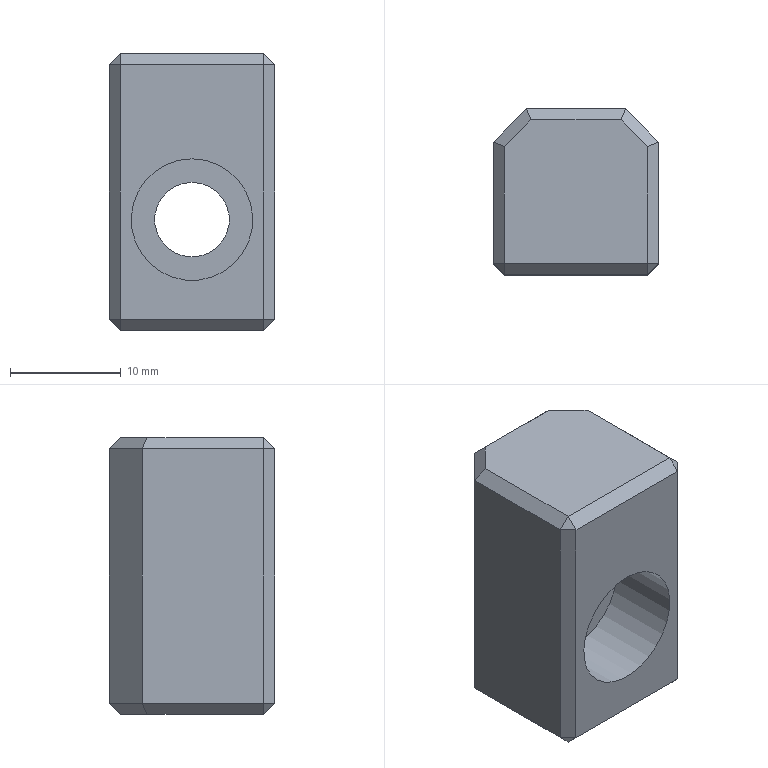Part | STEP file | solid 86 | 1 solid | 29 faces | box 15 x 15 x 25 mm | volume 4386 mm3 | plane 27 | cylinder 2 | commonest cylinder face diameters 6.75 x1 11 x1